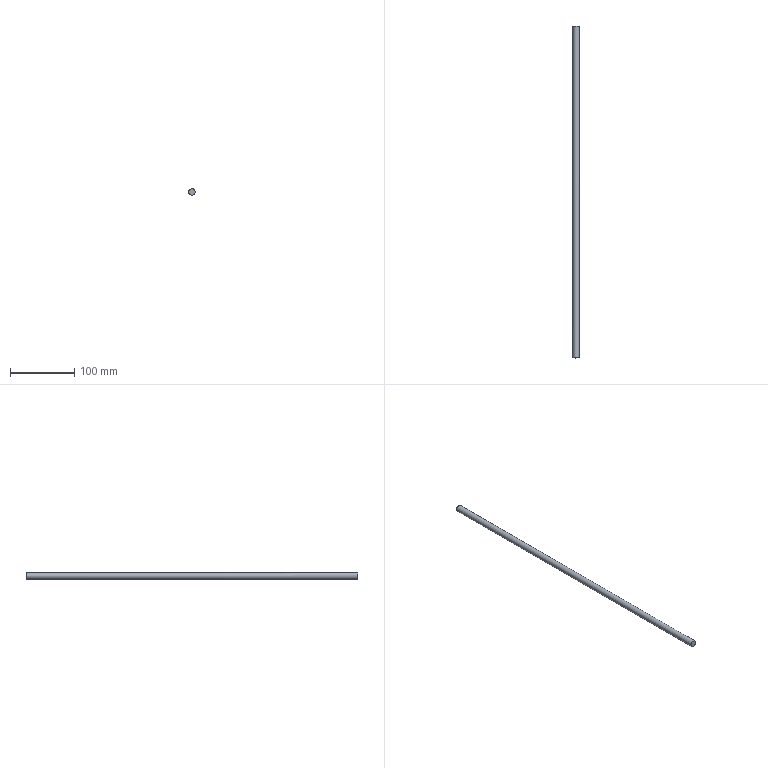Part | NX | features solid 2 | 1 solid | 3 faces | box 10 x 518 x 10 mm | volume 40684 mm3 | plane 2 | cylinder 1 | commonest cylinder face diameters 10 x1
STEP:
#1=CARTESIAN_POINT('',(371.,380.,-177.));
#2=VERTEX_POINT('',#1);
#3=CARTESIAN_POINT('',(371.,380.,-172.));
#4=DIRECTION('',(0.,-1.,0.));
#5=DIRECTION('',(0.,0.,-1.));
#6=AXIS2_PLACEMENT_3D('',#3,#4,#5);
#7=CIRCLE('',#6,5.);
#8=EDGE_CURVE('',#2,#2,#7,.T.);
#9=ORIENTED_EDGE('',*,*,#8,.T.);
#10=EDGE_LOOP('',(#9));
#11=FACE_BOUND('',#10,.T.);
#12=CARTESIAN_POINT('',(376.,-138.,-172.));
#13=VERTEX_POINT('',#12);
#14=CARTESIAN_POINT('',(371.,-138.,-172.));
#15=DIRECTION('',(0.,-1.,0.));
#16=DIRECTION('',(1.,0.,0.));
#17=AXIS2_PLACEMENT_3D('',#14,#15,#16);
#18=CIRCLE('',#17,5.);
#19=EDGE_CURVE('',#13,#13,#18,.T.);
#20=ORIENTED_EDGE('',*,*,#19,.F.);
#21=EDGE_LOOP('',(#20));
#22=FACE_BOUND('',#21,.T.);
#23=CARTESIAN_POINT('',(371.,862.5,-172.));
#24=DIRECTION('',(0.,-1.,0.));
#25=DIRECTION('',(0.,0.,-1.));
#26=AXIS2_PLACEMENT_3D('',#23,#24,#25);
#27=CYLINDRICAL_SURFACE('',#26,5.);
#28=ADVANCED_FACE('',(#11,#22),#27,.T.);
#29=ORIENTED_EDGE('',*,*,#8,.F.);
#30=EDGE_LOOP('',(#29));
#31=FACE_BOUND('',#30,.T.);
#32=CARTESIAN_POINT('',(120.,380.,-120.));
#33=DIRECTION('',(0.,-1.,0.));
#34=DIRECTION('',(0.,0.,-1.));
#35=AXIS2_PLACEMENT_3D('',#32,#33,#34);
#36=PLANE('',#35);
#37=ADVANCED_FACE('',(#31),#36,.F.);
#38=ORIENTED_EDGE('',*,*,#19,.T.);
#39=EDGE_LOOP('',(#38));
#40=FACE_BOUND('',#39,.T.);
#41=CARTESIAN_POINT('',(358.,-138.,-137.));
#42=DIRECTION('',(0.,-1.,0.));
#43=DIRECTION('',(1.,0.,0.));
#44=AXIS2_PLACEMENT_3D('',#41,#42,#43);
#45=PLANE('',#44);
#46=ADVANCED_FACE('',(#40),#45,.T.);
#47=CLOSED_SHELL('',(#28,#37,#46));
#48=MANIFOLD_SOLID_BREP('',#47);
#49=(LENGTH_UNIT()NAMED_UNIT(*)SI_UNIT(.MILLI.,.METRE.));
#50=UNCERTAINTY_MEASURE_WITH_UNIT(LENGTH_MEASURE(0.00001),#49,'','');
#51=(NAMED_UNIT(*)PLANE_ANGLE_UNIT()SI_UNIT($,.RADIAN.));
#52=(NAMED_UNIT(*)SI_UNIT($,.STERADIAN.)SOLID_ANGLE_UNIT());
#53=(GEOMETRIC_REPRESENTATION_CONTEXT(3)GLOBAL_UNCERTAINTY_ASSIGNED_CONTEXT((#50))GLOBAL_UNIT_ASSIGNED_CONTEXT((#49,#51,#52))REPRESENTATION_CONTEXT('',''));
#54=ADVANCED_BREP_SHAPE_REPRESENTATION('',(#48),#53);